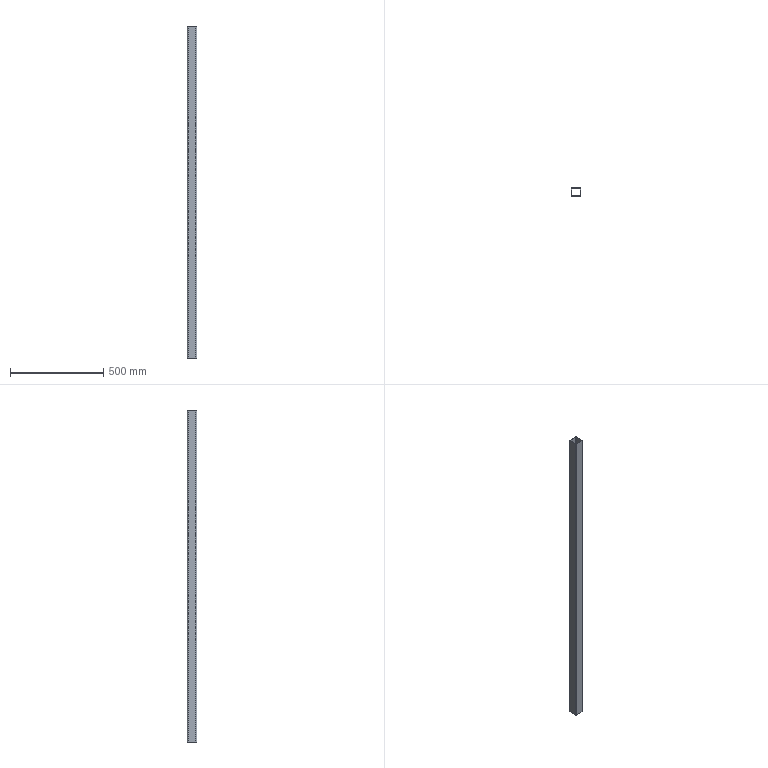Part | SolidWorks | features BaseBody 1 | 1 solid | 18 faces | box 50 x 50 x 1776 mm | volume 978796 mm3 | plane 10 | cylinder 8 | commonest cylinder face diameters 2 x4 8 x4
STEP:
#1=CARTESIAN_POINT('',(-22.,21.,-888.));
#2=VERTEX_POINT('',#1);
#3=CARTESIAN_POINT('',(-22.,-21.,-888.));
#4=VERTEX_POINT('',#3);
#5=CARTESIAN_POINT('',(-22.,21.,-888.));
#6=DIRECTION('',(0.,-1.,0.));
#7=VECTOR('',#6,1000.);
#8=LINE('',#5,#7);
#9=EDGE_CURVE('',#2,#4,#8,.T.);
#10=ORIENTED_EDGE('',*,*,#9,.F.);
#11=CARTESIAN_POINT('',(-22.,21.,888.));
#12=VERTEX_POINT('',#11);
#13=CARTESIAN_POINT('',(-22.,21.,888.));
#14=DIRECTION('',(0.,0.,-1.));
#15=VECTOR('',#14,1000.);
#16=LINE('',#13,#15);
#17=EDGE_CURVE('',#12,#2,#16,.T.);
#18=ORIENTED_EDGE('',*,*,#17,.F.);
#19=CARTESIAN_POINT('',(-22.,-21.,888.));
#20=VERTEX_POINT('',#19);
#21=CARTESIAN_POINT('',(-22.,21.,888.));
#22=DIRECTION('',(0.,-1.,0.));
#23=VECTOR('',#22,1000.);
#24=LINE('',#21,#23);
#25=EDGE_CURVE('',#12,#20,#24,.T.);
#26=ORIENTED_EDGE('',*,*,#25,.T.);
#27=CARTESIAN_POINT('',(-22.,-21.,888.));
#28=DIRECTION('',(0.,0.,-1.));
#29=VECTOR('',#28,1000.);
#30=LINE('',#27,#29);
#31=EDGE_CURVE('',#20,#4,#30,.T.);
#32=ORIENTED_EDGE('',*,*,#31,.T.);
#33=EDGE_LOOP('',(#10,#18,#26,#32));
#34=FACE_OUTER_BOUND('',#33,.T.);
#35=CARTESIAN_POINT('',(-22.,21.,888.));
#36=DIRECTION('',(1.,0.,0.));
#37=DIRECTION('',(0.,1.,0.));
#38=AXIS2_PLACEMENT_3D('',#35,#36,#37);
#39=PLANE('',#38);
#40=ADVANCED_FACE('',(#34),#39,.T.);
#41=CARTESIAN_POINT('',(-21.,22.,-888.));
#42=VERTEX_POINT('',#41);
#43=CARTESIAN_POINT('',(-21.,21.,-888.));
#44=DIRECTION('',(0.,0.,1.));
#45=DIRECTION('',(1.,0.,0.));
#46=AXIS2_PLACEMENT_3D('',#43,#44,#45);
#47=CIRCLE('',#46,1.);
#48=EDGE_CURVE('',#42,#2,#47,.T.);
#49=ORIENTED_EDGE('',*,*,#48,.F.);
#50=CARTESIAN_POINT('',(-21.,22.,888.));
#51=VERTEX_POINT('',#50);
#52=CARTESIAN_POINT('',(-21.,22.,888.));
#53=DIRECTION('',(0.,0.,-1.));
#54=VECTOR('',#53,1000.);
#55=LINE('',#52,#54);
#56=EDGE_CURVE('',#51,#42,#55,.T.);
#57=ORIENTED_EDGE('',*,*,#56,.F.);
#58=CARTESIAN_POINT('',(-21.,21.,888.));
#59=DIRECTION('',(0.,0.,1.));
#60=DIRECTION('',(1.,0.,0.));
#61=AXIS2_PLACEMENT_3D('',#58,#59,#60);
#62=CIRCLE('',#61,1.);
#63=EDGE_CURVE('',#51,#12,#62,.T.);
#64=ORIENTED_EDGE('',*,*,#63,.T.);
#65=ORIENTED_EDGE('',*,*,#17,.T.);
#66=EDGE_LOOP('',(#49,#57,#64,#65));
#67=FACE_OUTER_BOUND('',#66,.T.);
#68=CARTESIAN_POINT('',(-21.,21.,888.));
#69=DIRECTION('',(0.,0.,-1.));
#70=DIRECTION('',(-1.,0.,0.));
#71=AXIS2_PLACEMENT_3D('',#68,#69,#70);
#72=CYLINDRICAL_SURFACE('',#71,1.);
#73=ADVANCED_FACE('',(#67),#72,.F.);
#74=CARTESIAN_POINT('',(21.,22.,-888.));
#75=VERTEX_POINT('',#74);
#76=CARTESIAN_POINT('',(-21.,22.,-888.));
#77=DIRECTION('',(-1.,0.,0.));
#78=VECTOR('',#77,1000.);
#79=LINE('',#76,#78);
#80=EDGE_CURVE('',#75,#42,#79,.T.);
#81=ORIENTED_EDGE('',*,*,#80,.F.);
#82=CARTESIAN_POINT('',(21.,22.,888.));
#83=VERTEX_POINT('',#82);
#84=CARTESIAN_POINT('',(21.,22.,888.));
#85=DIRECTION('',(0.,0.,-1.));
#86=VECTOR('',#85,1000.);
#87=LINE('',#84,#86);
#88=EDGE_CURVE('',#83,#75,#87,.T.);
#89=ORIENTED_EDGE('',*,*,#88,.F.);
#90=CARTESIAN_POINT('',(-21.,22.,888.));
#91=DIRECTION('',(-1.,0.,0.));
#92=VECTOR('',#91,1000.);
#93=LINE('',#90,#92);
#94=EDGE_CURVE('',#83,#51,#93,.T.);
#95=ORIENTED_EDGE('',*,*,#94,.T.);
#96=ORIENTED_EDGE('',*,*,#56,.T.);
#97=EDGE_LOOP('',(#81,#89,#95,#96));
#98=FACE_OUTER_BOUND('',#97,.T.);
#99=CARTESIAN_POINT('',(-21.,22.,888.));
#100=DIRECTION('',(0.,-1.,0.));
#101=DIRECTION('',(0.,0.,-1.));
#102=AXIS2_PLACEMENT_3D('',#99,#100,#101);
#103=PLANE('',#102);
#104=ADVANCED_FACE('',(#98),#103,.T.);
#105=CARTESIAN_POINT('',(22.,21.,-888.));
#106=VERTEX_POINT('',#105);
#107=CARTESIAN_POINT('',(21.,21.,-888.));
#108=DIRECTION('',(0.,0.,1.));
#109=DIRECTION('',(1.,0.,0.));
#110=AXIS2_PLACEMENT_3D('',#107,#108,#109);
#111=CIRCLE('',#110,1.);
#112=EDGE_CURVE('',#106,#75,#111,.T.);
#113=ORIENTED_EDGE('',*,*,#112,.F.);
#114=CARTESIAN_POINT('',(22.,21.,888.));
#115=VERTEX_POINT('',#114);
#116=CARTESIAN_POINT('',(22.,21.,888.));
#117=DIRECTION('',(0.,0.,-1.));
#118=VECTOR('',#117,1000.);
#119=LINE('',#116,#118);
#120=EDGE_CURVE('',#115,#106,#119,.T.);
#121=ORIENTED_EDGE('',*,*,#120,.F.);
#122=CARTESIAN_POINT('',(21.,21.,888.));
#123=DIRECTION('',(0.,0.,1.));
#124=DIRECTION('',(1.,0.,0.));
#125=AXIS2_PLACEMENT_3D('',#122,#123,#124);
#126=CIRCLE('',#125,1.);
#127=EDGE_CURVE('',#115,#83,#126,.T.);
#128=ORIENTED_EDGE('',*,*,#127,.T.);
#129=ORIENTED_EDGE('',*,*,#88,.T.);
#130=EDGE_LOOP('',(#113,#121,#128,#129));
#131=FACE_OUTER_BOUND('',#130,.T.);
#132=CARTESIAN_POINT('',(21.,21.,888.));
#133=DIRECTION('',(0.,0.,-1.));
#134=DIRECTION('',(-1.,0.,0.));
#135=AXIS2_PLACEMENT_3D('',#132,#133,#134);
#136=CYLINDRICAL_SURFACE('',#135,1.);
#137=ADVANCED_FACE('',(#131),#136,.F.);
#138=CARTESIAN_POINT('',(22.,-21.,-888.));
#139=VERTEX_POINT('',#138);
#140=CARTESIAN_POINT('',(22.,21.,-888.));
#141=DIRECTION('',(0.,1.,0.));
#142=VECTOR('',#141,1000.);
#143=LINE('',#140,#142);
#144=EDGE_CURVE('',#139,#106,#143,.T.);
#145=ORIENTED_EDGE('',*,*,#144,.F.);
#146=CARTESIAN_POINT('',(22.,-21.,888.));
#147=VERTEX_POINT('',#146);
#148=CARTESIAN_POINT('',(22.,-21.,888.));
#149=DIRECTION('',(0.,0.,-1.));
#150=VECTOR('',#149,1000.);
#151=LINE('',#148,#150);
#152=EDGE_CURVE('',#147,#139,#151,.T.);
#153=ORIENTED_EDGE('',*,*,#152,.F.);
#154=CARTESIAN_POINT('',(22.,21.,888.));
#155=DIRECTION('',(0.,1.,0.));
#156=VECTOR('',#155,1000.);
#157=LINE('',#154,#156);
#158=EDGE_CURVE('',#147,#115,#157,.T.);
#159=ORIENTED_EDGE('',*,*,#158,.T.);
#160=ORIENTED_EDGE('',*,*,#120,.T.);
#161=EDGE_LOOP('',(#145,#153,#159,#160));
#162=FACE_OUTER_BOUND('',#161,.T.);
#163=CARTESIAN_POINT('',(22.,21.,888.));
#164=DIRECTION('',(-1.,0.,0.));
#165=DIRECTION('',(0.,1.,0.));
#166=AXIS2_PLACEMENT_3D('',#163,#164,#165);
#167=PLANE('',#166);
#168=ADVANCED_FACE('',(#162),#167,.T.);
#169=CARTESIAN_POINT('',(21.,-22.,-888.));
#170=VERTEX_POINT('',#169);
#171=CARTESIAN_POINT('',(21.,-21.,-888.));
#172=DIRECTION('',(0.,0.,1.));
#173=DIRECTION('',(1.,0.,0.));
#174=AXIS2_PLACEMENT_3D('',#171,#172,#173);
#175=CIRCLE('',#174,1.);
#176=EDGE_CURVE('',#170,#139,#175,.T.);
#177=ORIENTED_EDGE('',*,*,#176,.F.);
#178=CARTESIAN_POINT('',(21.,-22.,888.));
#179=VERTEX_POINT('',#178);
#180=CARTESIAN_POINT('',(21.,-22.,888.));
#181=DIRECTION('',(0.,0.,-1.));
#182=VECTOR('',#181,1000.);
#183=LINE('',#180,#182);
#184=EDGE_CURVE('',#179,#170,#183,.T.);
#185=ORIENTED_EDGE('',*,*,#184,.F.);
#186=CARTESIAN_POINT('',(21.,-21.,888.));
#187=DIRECTION('',(0.,0.,1.));
#188=DIRECTION('',(1.,0.,0.));
#189=AXIS2_PLACEMENT_3D('',#186,#187,#188);
#190=CIRCLE('',#189,1.);
#191=EDGE_CURVE('',#179,#147,#190,.T.);
#192=ORIENTED_EDGE('',*,*,#191,.T.);
#193=ORIENTED_EDGE('',*,*,#152,.T.);
#194=EDGE_LOOP('',(#177,#185,#192,#193));
#195=FACE_OUTER_BOUND('',#194,.T.);
#196=CARTESIAN_POINT('',(21.,-21.,888.));
#197=DIRECTION('',(0.,0.,-1.));
#198=DIRECTION('',(-1.,0.,0.));
#199=AXIS2_PLACEMENT_3D('',#196,#197,#198);
#200=CYLINDRICAL_SURFACE('',#199,1.);
#201=ADVANCED_FACE('',(#195),#200,.F.);
#202=CARTESIAN_POINT('',(-21.,-22.,-888.));
#203=VERTEX_POINT('',#202);
#204=CARTESIAN_POINT('',(-21.,-22.,-888.));
#205=DIRECTION('',(1.,0.,0.));
#206=VECTOR('',#205,1000.);
#207=LINE('',#204,#206);
#208=EDGE_CURVE('',#203,#170,#207,.T.);
#209=ORIENTED_EDGE('',*,*,#208,.F.);
#210=CARTESIAN_POINT('',(-21.,-22.,888.));
#211=VERTEX_POINT('',#210);
#212=CARTESIAN_POINT('',(-21.,-22.,888.));
#213=DIRECTION('',(0.,0.,-1.));
#214=VECTOR('',#213,1000.);
#215=LINE('',#212,#214);
#216=EDGE_CURVE('',#211,#203,#215,.T.);
#217=ORIENTED_EDGE('',*,*,#216,.F.);
#218=CARTESIAN_POINT('',(-21.,-22.,888.));
#219=DIRECTION('',(1.,0.,0.));
#220=VECTOR('',#219,1000.);
#221=LINE('',#218,#220);
#222=EDGE_CURVE('',#211,#179,#221,.T.);
#223=ORIENTED_EDGE('',*,*,#222,.T.);
#224=ORIENTED_EDGE('',*,*,#184,.T.);
#225=EDGE_LOOP('',(#209,#217,#223,#224));
#226=FACE_OUTER_BOUND('',#225,.T.);
#227=CARTESIAN_POINT('',(-21.,-22.,888.));
#228=DIRECTION('',(0.,1.,0.));
#229=DIRECTION('',(1.,0.,0.));
#230=AXIS2_PLACEMENT_3D('',#227,#228,#229);
#231=PLANE('',#230);
#232=ADVANCED_FACE('',(#226),#231,.T.);
#233=CARTESIAN_POINT('',(-21.,-21.,-888.));
#234=DIRECTION('',(0.,0.,1.));
#235=DIRECTION('',(1.,0.,0.));
#236=AXIS2_PLACEMENT_3D('',#233,#234,#235);
#237=CIRCLE('',#236,1.);
#238=EDGE_CURVE('',#4,#203,#237,.T.);
#239=ORIENTED_EDGE('',*,*,#238,.F.);
#240=ORIENTED_EDGE('',*,*,#31,.F.);
#241=CARTESIAN_POINT('',(-21.,-21.,888.));
#242=DIRECTION('',(0.,0.,1.));
#243=DIRECTION('',(1.,0.,0.));
#244=AXIS2_PLACEMENT_3D('',#241,#242,#243);
#245=CIRCLE('',#244,1.);
#246=EDGE_CURVE('',#20,#211,#245,.T.);
#247=ORIENTED_EDGE('',*,*,#246,.T.);
#248=ORIENTED_EDGE('',*,*,#216,.T.);
#249=EDGE_LOOP('',(#239,#240,#247,#248));
#250=FACE_OUTER_BOUND('',#249,.T.);
#251=CARTESIAN_POINT('',(-21.,-21.,888.));
#252=DIRECTION('',(0.,0.,-1.));
#253=DIRECTION('',(-1.,0.,0.));
#254=AXIS2_PLACEMENT_3D('',#251,#252,#253);
#255=CYLINDRICAL_SURFACE('',#254,1.);
#256=ADVANCED_FACE('',(#250),#255,.F.);
#257=CARTESIAN_POINT('',(-25.,21.,-888.));
#258=VERTEX_POINT('',#257);
#259=CARTESIAN_POINT('',(-25.,-21.,-888.));
#260=VERTEX_POINT('',#259);
#261=CARTESIAN_POINT('',(-25.,21.,-888.));
#262=DIRECTION('',(0.,-1.,0.));
#263=VECTOR('',#262,1000.);
#264=LINE('',#261,#263);
#265=EDGE_CURVE('',#258,#260,#264,.T.);
#266=ORIENTED_EDGE('',*,*,#265,.T.);
#267=CARTESIAN_POINT('',(-25.,-21.,888.));
#268=VERTEX_POINT('',#267);
#269=CARTESIAN_POINT('',(-25.,-21.,888.));
#270=DIRECTION('',(0.,0.,-1.));
#271=VECTOR('',#270,1000.);
#272=LINE('',#269,#271);
#273=EDGE_CURVE('',#268,#260,#272,.T.);
#274=ORIENTED_EDGE('',*,*,#273,.F.);
#275=CARTESIAN_POINT('',(-25.,21.,888.));
#276=VERTEX_POINT('',#275);
#277=CARTESIAN_POINT('',(-25.,21.,888.));
#278=DIRECTION('',(0.,-1.,0.));
#279=VECTOR('',#278,1000.);
#280=LINE('',#277,#279);
#281=EDGE_CURVE('',#276,#268,#280,.T.);
#282=ORIENTED_EDGE('',*,*,#281,.F.);
#283=CARTESIAN_POINT('',(-25.,21.,888.));
#284=DIRECTION('',(0.,0.,-1.));
#285=VECTOR('',#284,1000.);
#286=LINE('',#283,#285);
#287=EDGE_CURVE('',#276,#258,#286,.T.);
#288=ORIENTED_EDGE('',*,*,#287,.T.);
#289=EDGE_LOOP('',(#266,#274,#282,#288));
#290=FACE_OUTER_BOUND('',#289,.T.);
#291=CARTESIAN_POINT('',(-25.,21.,888.));
#292=DIRECTION('',(1.,0.,0.));
#293=DIRECTION('',(0.,1.,0.));
#294=AXIS2_PLACEMENT_3D('',#291,#292,#293);
#295=PLANE('',#294);
#296=ADVANCED_FACE('',(#290),#295,.F.);
#297=CARTESIAN_POINT('',(-21.,25.,-888.));
#298=VERTEX_POINT('',#297);
#299=CARTESIAN_POINT('',(-21.,21.,-888.));
#300=DIRECTION('',(0.,0.,1.));
#301=DIRECTION('',(1.,0.,0.));
#302=AXIS2_PLACEMENT_3D('',#299,#300,#301);
#303=CIRCLE('',#302,4.);
#304=EDGE_CURVE('',#298,#258,#303,.T.);
#305=ORIENTED_EDGE('',*,*,#304,.T.);
#306=ORIENTED_EDGE('',*,*,#287,.F.);
#307=CARTESIAN_POINT('',(-21.,25.,888.));
#308=VERTEX_POINT('',#307);
#309=CARTESIAN_POINT('',(-21.,21.,888.));
#310=DIRECTION('',(0.,0.,1.));
#311=DIRECTION('',(1.,0.,0.));
#312=AXIS2_PLACEMENT_3D('',#309,#310,#311);
#313=CIRCLE('',#312,4.);
#314=EDGE_CURVE('',#308,#276,#313,.T.);
#315=ORIENTED_EDGE('',*,*,#314,.F.);
#316=CARTESIAN_POINT('',(-21.,25.,888.));
#317=DIRECTION('',(0.,0.,-1.));
#318=VECTOR('',#317,1000.);
#319=LINE('',#316,#318);
#320=EDGE_CURVE('',#308,#298,#319,.T.);
#321=ORIENTED_EDGE('',*,*,#320,.T.);
#322=EDGE_LOOP('',(#305,#306,#315,#321));
#323=FACE_OUTER_BOUND('',#322,.T.);
#324=CARTESIAN_POINT('',(-21.,21.,888.));
#325=DIRECTION('',(0.,0.,-1.));
#326=DIRECTION('',(-1.,0.,0.));
#327=AXIS2_PLACEMENT_3D('',#324,#325,#326);
#328=CYLINDRICAL_SURFACE('',#327,4.);
#329=ADVANCED_FACE('',(#323),#328,.T.);
#330=CARTESIAN_POINT('',(21.,25.,-888.));
#331=VERTEX_POINT('',#330);
#332=CARTESIAN_POINT('',(-21.,25.,-888.));
#333=DIRECTION('',(-1.,0.,0.));
#334=VECTOR('',#333,1000.);
#335=LINE('',#332,#334);
#336=EDGE_CURVE('',#331,#298,#335,.T.);
#337=ORIENTED_EDGE('',*,*,#336,.T.);
#338=ORIENTED_EDGE('',*,*,#320,.F.);
#339=CARTESIAN_POINT('',(21.,25.,888.));
#340=VERTEX_POINT('',#339);
#341=CARTESIAN_POINT('',(-21.,25.,888.));
#342=DIRECTION('',(-1.,0.,0.));
#343=VECTOR('',#342,1000.);
#344=LINE('',#341,#343);
#345=EDGE_CURVE('',#340,#308,#344,.T.);
#346=ORIENTED_EDGE('',*,*,#345,.F.);
#347=CARTESIAN_POINT('',(21.,25.,888.));
#348=DIRECTION('',(0.,0.,-1.));
#349=VECTOR('',#348,1000.);
#350=LINE('',#347,#349);
#351=EDGE_CURVE('',#340,#331,#350,.T.);
#352=ORIENTED_EDGE('',*,*,#351,.T.);
#353=EDGE_LOOP('',(#337,#338,#346,#352));
#354=FACE_OUTER_BOUND('',#353,.T.);
#355=CARTESIAN_POINT('',(-21.,25.,888.));
#356=DIRECTION('',(0.,-1.,0.));
#357=DIRECTION('',(0.,0.,-1.));
#358=AXIS2_PLACEMENT_3D('',#355,#356,#357);
#359=PLANE('',#358);
#360=ADVANCED_FACE('',(#354),#359,.F.);
#361=CARTESIAN_POINT('',(25.,21.,-888.));
#362=VERTEX_POINT('',#361);
#363=CARTESIAN_POINT('',(21.,21.,-888.));
#364=DIRECTION('',(0.,0.,1.));
#365=DIRECTION('',(-1.,0.,0.));
#366=AXIS2_PLACEMENT_3D('',#363,#364,#365);
#367=CIRCLE('',#366,4.);
#368=EDGE_CURVE('',#362,#331,#367,.T.);
#369=ORIENTED_EDGE('',*,*,#368,.T.);
#370=ORIENTED_EDGE('',*,*,#351,.F.);
#371=CARTESIAN_POINT('',(25.,21.,888.));
#372=VERTEX_POINT('',#371);
#373=CARTESIAN_POINT('',(21.,21.,888.));
#374=DIRECTION('',(0.,0.,1.));
#375=DIRECTION('',(-1.,0.,0.));
#376=AXIS2_PLACEMENT_3D('',#373,#374,#375);
#377=CIRCLE('',#376,4.);
#378=EDGE_CURVE('',#372,#340,#377,.T.);
#379=ORIENTED_EDGE('',*,*,#378,.F.);
#380=CARTESIAN_POINT('',(25.,21.,888.));
#381=DIRECTION('',(0.,0.,-1.));
#382=VECTOR('',#381,1000.);
#383=LINE('',#380,#382);
#384=EDGE_CURVE('',#372,#362,#383,.T.);
#385=ORIENTED_EDGE('',*,*,#384,.T.);
#386=EDGE_LOOP('',(#369,#370,#379,#385));
#387=FACE_OUTER_BOUND('',#386,.T.);
#388=CARTESIAN_POINT('',(21.,21.,888.));
#389=DIRECTION('',(0.,0.,-1.));
#390=DIRECTION('',(-1.,0.,0.));
#391=AXIS2_PLACEMENT_3D('',#388,#389,#390);
#392=CYLINDRICAL_SURFACE('',#391,4.);
#393=ADVANCED_FACE('',(#387),#392,.T.);
#394=CARTESIAN_POINT('',(25.,-21.,-888.));
#395=VERTEX_POINT('',#394);
#396=CARTESIAN_POINT('',(25.,21.,-888.));
#397=DIRECTION('',(0.,1.,0.));
#398=VECTOR('',#397,1000.);
#399=LINE('',#396,#398);
#400=EDGE_CURVE('',#395,#362,#399,.T.);
#401=ORIENTED_EDGE('',*,*,#400,.T.);
#402=ORIENTED_EDGE('',*,*,#384,.F.);
#403=CARTESIAN_POINT('',(25.,-21.,888.));
#404=VERTEX_POINT('',#403);
#405=CARTESIAN_POINT('',(25.,21.,888.));
#406=DIRECTION('',(0.,1.,0.));
#407=VECTOR('',#406,1000.);
#408=LINE('',#405,#407);
#409=EDGE_CURVE('',#404,#372,#408,.T.);
#410=ORIENTED_EDGE('',*,*,#409,.F.);
#411=CARTESIAN_POINT('',(25.,-21.,888.));
#412=DIRECTION('',(0.,0.,-1.));
#413=VECTOR('',#412,1000.);
#414=LINE('',#411,#413);
#415=EDGE_CURVE('',#404,#395,#414,.T.);
#416=ORIENTED_EDGE('',*,*,#415,.T.);
#417=EDGE_LOOP('',(#401,#402,#410,#416));
#418=FACE_OUTER_BOUND('',#417,.T.);
#419=CARTESIAN_POINT('',(25.,21.,888.));
#420=DIRECTION('',(-1.,0.,0.));
#421=DIRECTION('',(0.,1.,0.));
#422=AXIS2_PLACEMENT_3D('',#419,#420,#421);
#423=PLANE('',#422);
#424=ADVANCED_FACE('',(#418),#423,.F.);
#425=CARTESIAN_POINT('',(21.,-25.,-888.));
#426=VERTEX_POINT('',#425);
#427=CARTESIAN_POINT('',(21.,-21.,-888.));
#428=DIRECTION('',(0.,0.,1.));
#429=DIRECTION('',(1.,0.,0.));
#430=AXIS2_PLACEMENT_3D('',#427,#428,#429);
#431=CIRCLE('',#430,4.);
#432=EDGE_CURVE('',#426,#395,#431,.T.);
#433=ORIENTED_EDGE('',*,*,#432,.T.);
#434=ORIENTED_EDGE('',*,*,#415,.F.);
#435=CARTESIAN_POINT('',(21.,-25.,888.));
#436=VERTEX_POINT('',#435);
#437=CARTESIAN_POINT('',(21.,-21.,888.));
#438=DIRECTION('',(0.,0.,1.));
#439=DIRECTION('',(1.,0.,0.));
#440=AXIS2_PLACEMENT_3D('',#437,#438,#439);
#441=CIRCLE('',#440,4.);
#442=EDGE_CURVE('',#436,#404,#441,.T.);
#443=ORIENTED_EDGE('',*,*,#442,.F.);
#444=CARTESIAN_POINT('',(21.,-25.,888.));
#445=DIRECTION('',(0.,0.,-1.));
#446=VECTOR('',#445,1000.);
#447=LINE('',#444,#446);
#448=EDGE_CURVE('',#436,#426,#447,.T.);
#449=ORIENTED_EDGE('',*,*,#448,.T.);
#450=EDGE_LOOP('',(#433,#434,#443,#449));
#451=FACE_OUTER_BOUND('',#450,.T.);
#452=CARTESIAN_POINT('',(21.,-21.,888.));
#453=DIRECTION('',(0.,0.,-1.));
#454=DIRECTION('',(-1.,0.,0.));
#455=AXIS2_PLACEMENT_3D('',#452,#453,#454);
#456=CYLINDRICAL_SURFACE('',#455,4.);
#457=ADVANCED_FACE('',(#451),#456,.T.);
#458=CARTESIAN_POINT('',(-21.,-25.,-888.));
#459=VERTEX_POINT('',#458);
#460=CARTESIAN_POINT('',(-21.,-25.,-888.));
#461=DIRECTION('',(1.,0.,0.));
#462=VECTOR('',#461,1000.);
#463=LINE('',#460,#462);
#464=EDGE_CURVE('',#459,#426,#463,.T.);
#465=ORIENTED_EDGE('',*,*,#464,.T.);
#466=ORIENTED_EDGE('',*,*,#448,.F.);
#467=CARTESIAN_POINT('',(-21.,-25.,888.));
#468=VERTEX_POINT('',#467);
#469=CARTESIAN_POINT('',(-21.,-25.,888.));
#470=DIRECTION('',(1.,0.,0.));
#471=VECTOR('',#470,1000.);
#472=LINE('',#469,#471);
#473=EDGE_CURVE('',#468,#436,#472,.T.);
#474=ORIENTED_EDGE('',*,*,#473,.F.);
#475=CARTESIAN_POINT('',(-21.,-25.,888.));
#476=DIRECTION('',(0.,0.,-1.));
#477=VECTOR('',#476,1000.);
#478=LINE('',#475,#477);
#479=EDGE_CURVE('',#468,#459,#478,.T.);
#480=ORIENTED_EDGE('',*,*,#479,.T.);
#481=EDGE_LOOP('',(#465,#466,#474,#480));
#482=FACE_OUTER_BOUND('',#481,.T.);
#483=CARTESIAN_POINT('',(-21.,-25.,888.));
#484=DIRECTION('',(0.,1.,0.));
#485=DIRECTION('',(1.,0.,0.));
#486=AXIS2_PLACEMENT_3D('',#483,#484,#485);
#487=PLANE('',#486);
#488=ADVANCED_FACE('',(#482),#487,.F.);
#489=CARTESIAN_POINT('',(-21.,-21.,-888.));
#490=DIRECTION('',(0.,0.,1.));
#491=DIRECTION('',(1.,0.,0.));
#492=AXIS2_PLACEMENT_3D('',#489,#490,#491);
#493=CIRCLE('',#492,4.);
#494=EDGE_CURVE('',#260,#459,#493,.T.);
#495=ORIENTED_EDGE('',*,*,#494,.T.);
#496=ORIENTED_EDGE('',*,*,#479,.F.);
#497=CARTESIAN_POINT('',(-21.,-21.,888.));
#498=DIRECTION('',(0.,0.,1.));
#499=DIRECTION('',(1.,0.,0.));
#500=AXIS2_PLACEMENT_3D('',#497,#498,#499);
#501=CIRCLE('',#500,4.);
#502=EDGE_CURVE('',#268,#468,#501,.T.);
#503=ORIENTED_EDGE('',*,*,#502,.F.);
#504=ORIENTED_EDGE('',*,*,#273,.T.);
#505=EDGE_LOOP('',(#495,#496,#503,#504));
#506=FACE_OUTER_BOUND('',#505,.T.);
#507=CARTESIAN_POINT('',(-21.,-21.,888.));
#508=DIRECTION('',(0.,0.,-1.));
#509=DIRECTION('',(-1.,0.,0.));
#510=AXIS2_PLACEMENT_3D('',#507,#508,#509);
#511=CYLINDRICAL_SURFACE('',#510,4.);
#512=ADVANCED_FACE('',(#506),#511,.T.);
#513=ORIENTED_EDGE('',*,*,#238,.T.);
#514=ORIENTED_EDGE('',*,*,#208,.T.);
#515=ORIENTED_EDGE('',*,*,#176,.T.);
#516=ORIENTED_EDGE('',*,*,#144,.T.);
#517=ORIENTED_EDGE('',*,*,#112,.T.);
#518=ORIENTED_EDGE('',*,*,#80,.T.);
#519=ORIENTED_EDGE('',*,*,#48,.T.);
#520=ORIENTED_EDGE('',*,*,#9,.T.);
#521=EDGE_LOOP('',(#513,#514,#515,#516,#517,#518,#519,#520));
#522=FACE_BOUND('',#521,.T.);
#523=ORIENTED_EDGE('',*,*,#494,.F.);
#524=ORIENTED_EDGE('',*,*,#265,.F.);
#525=ORIENTED_EDGE('',*,*,#304,.F.);
#526=ORIENTED_EDGE('',*,*,#336,.F.);
#527=ORIENTED_EDGE('',*,*,#368,.F.);
#528=ORIENTED_EDGE('',*,*,#400,.F.);
#529=ORIENTED_EDGE('',*,*,#432,.F.);
#530=ORIENTED_EDGE('',*,*,#464,.F.);
#531=EDGE_LOOP('',(#523,#524,#525,#526,#527,#528,#529,#530));
#532=FACE_OUTER_BOUND('',#531,.T.);
#533=CARTESIAN_POINT('',(-21.,-21.,-888.));
#534=DIRECTION('',(0.,0.,1.));
#535=DIRECTION('',(1.,0.,0.));
#536=AXIS2_PLACEMENT_3D('',#533,#534,#535);
#537=PLANE('',#536);
#538=ADVANCED_FACE('',(#522,#532),#537,.F.);
#539=ORIENTED_EDGE('',*,*,#222,.F.);
#540=ORIENTED_EDGE('',*,*,#246,.F.);
#541=ORIENTED_EDGE('',*,*,#25,.F.);
#542=ORIENTED_EDGE('',*,*,#63,.F.);
#543=ORIENTED_EDGE('',*,*,#94,.F.);
#544=ORIENTED_EDGE('',*,*,#127,.F.);
#545=ORIENTED_EDGE('',*,*,#158,.F.);
#546=ORIENTED_EDGE('',*,*,#191,.F.);
#547=EDGE_LOOP('',(#539,#540,#541,#542,#543,#544,#545,#546));
#548=FACE_BOUND('',#547,.T.);
#549=ORIENTED_EDGE('',*,*,#502,.T.);
#550=ORIENTED_EDGE('',*,*,#473,.T.);
#551=ORIENTED_EDGE('',*,*,#442,.T.);
#552=ORIENTED_EDGE('',*,*,#409,.T.);
#553=ORIENTED_EDGE('',*,*,#378,.T.);
#554=ORIENTED_EDGE('',*,*,#345,.T.);
#555=ORIENTED_EDGE('',*,*,#314,.T.);
#556=ORIENTED_EDGE('',*,*,#281,.T.);
#557=EDGE_LOOP('',(#549,#550,#551,#552,#553,#554,#555,#556));
#558=FACE_OUTER_BOUND('',#557,.T.);
#559=CARTESIAN_POINT('',(-21.,-21.,888.));
#560=DIRECTION('',(0.,0.,1.));
#561=DIRECTION('',(1.,0.,0.));
#562=AXIS2_PLACEMENT_3D('',#559,#560,#561);
#563=PLANE('',#562);
#564=ADVANCED_FACE('',(#548,#558),#563,.T.);
#565=CLOSED_SHELL('',(#40,#73,#104,#137,#168,#201,#232,#256,#296,#329,#360,#393,#424,#457,#488,#512,#538,#564));
#566=MANIFOLD_SOLID_BREP('',#565);
#567=CARTESIAN_POINT('',(0.,0.,0.));
#568=DIRECTION('',(0.,0.,1.));
#569=DIRECTION('',(1.,0.,0.));
#570=AXIS2_PLACEMENT_3D('',#567,#568,#569);
#571=(LENGTH_UNIT()NAMED_UNIT(*)SI_UNIT(.MILLI.,.METRE.));
#572=UNCERTAINTY_MEASURE_WITH_UNIT(LENGTH_MEASURE(0.00001),#571,'','');
#573=(NAMED_UNIT(*)PLANE_ANGLE_UNIT()SI_UNIT($,.RADIAN.));
#574=(NAMED_UNIT(*)SI_UNIT($,.STERADIAN.)SOLID_ANGLE_UNIT());
#575=(GEOMETRIC_REPRESENTATION_CONTEXT(3)GLOBAL_UNCERTAINTY_ASSIGNED_CONTEXT((#572))GLOBAL_UNIT_ASSIGNED_CONTEXT((#571,#573,#574))REPRESENTATION_CONTEXT('',''));
#576=ADVANCED_BREP_SHAPE_REPRESENTATION('',(#566,#570),#575);